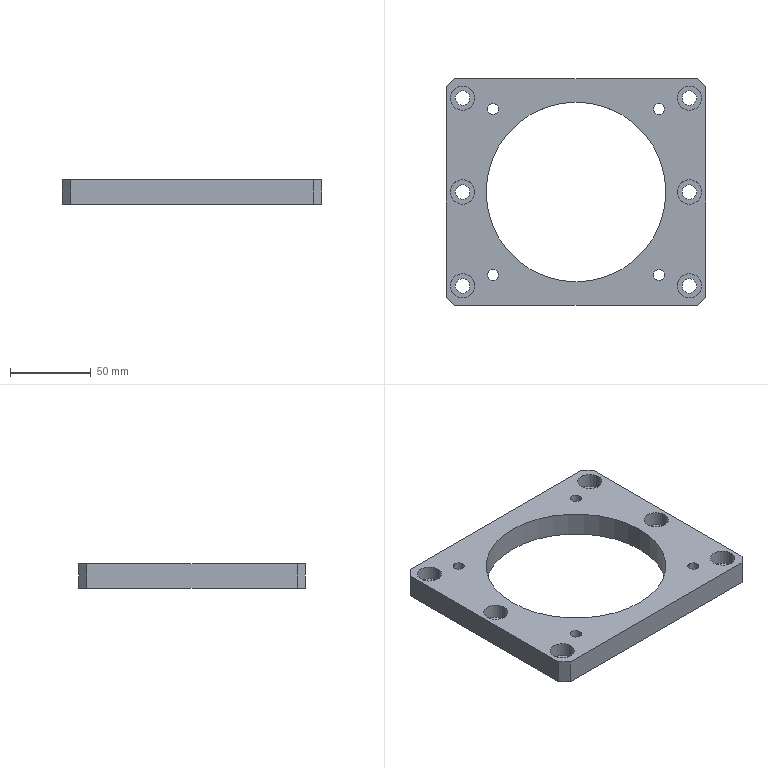Part | SolidWorks | features HoleWzd 2, CirPattern 1, Extrusion 1, MirrorPattern 1 | 1 solid | 50 faces | box 160 x 140 x 15 mm | volume 176085 mm3 | cylinder 34 | plane 16 | commonest cylinder face diameters 9 x12 15 x12 6.8 x8 111 x2
STEP:
#1=CARTESIAN_POINT('',(-77.5,58.,6.));
#2=VERTEX_POINT('',#1);
#3=CARTESIAN_POINT('',(-62.5,58.,6.));
#4=VERTEX_POINT('',#3);
#5=CARTESIAN_POINT('',(-70.,58.,6.));
#6=DIRECTION('',(0.,0.,1.));
#7=DIRECTION('',(1.,0.,0.));
#8=AXIS2_PLACEMENT_3D('',#5,#6,#7);
#9=CIRCLE('',#8,7.5);
#10=EDGE_CURVE('',#2,#4,#9,.T.);
#11=ORIENTED_EDGE('',*,*,#10,.F.);
#12=CARTESIAN_POINT('',(-77.5,58.,15.));
#13=VERTEX_POINT('',#12);
#14=CARTESIAN_POINT('',(-77.5,58.,15.));
#15=DIRECTION('',(0.,0.,1.));
#16=VECTOR('',#15,1000.);
#17=LINE('',#14,#16);
#18=EDGE_CURVE('',#2,#13,#17,.T.);
#19=ORIENTED_EDGE('',*,*,#18,.T.);
#20=CARTESIAN_POINT('',(-62.5,58.,15.));
#21=VERTEX_POINT('',#20);
#22=CARTESIAN_POINT('',(-70.,58.,15.));
#23=DIRECTION('',(0.,0.,1.));
#24=DIRECTION('',(1.,0.,0.));
#25=AXIS2_PLACEMENT_3D('',#22,#23,#24);
#26=CIRCLE('',#25,7.5);
#27=EDGE_CURVE('',#13,#21,#26,.T.);
#28=ORIENTED_EDGE('',*,*,#27,.T.);
#29=CARTESIAN_POINT('',(-62.5,58.,15.));
#30=DIRECTION('',(0.,0.,1.));
#31=VECTOR('',#30,1000.);
#32=LINE('',#29,#31);
#33=EDGE_CURVE('',#4,#21,#32,.T.);
#34=ORIENTED_EDGE('',*,*,#33,.F.);
#35=EDGE_LOOP('',(#11,#19,#28,#34));
#36=FACE_OUTER_BOUND('',#35,.T.);
#37=CARTESIAN_POINT('',(-70.,58.,15.));
#38=DIRECTION('',(0.,0.,1.));
#39=DIRECTION('',(1.,0.,0.));
#40=AXIS2_PLACEMENT_3D('',#37,#38,#39);
#41=CYLINDRICAL_SURFACE('',#40,7.5);
#42=ADVANCED_FACE('',(#36),#41,.F.);
#43=CARTESIAN_POINT('',(-74.5,58.,0.));
#44=VERTEX_POINT('',#43);
#45=CARTESIAN_POINT('',(-65.5,58.,0.));
#46=VERTEX_POINT('',#45);
#47=CARTESIAN_POINT('',(-70.,58.,0.));
#48=DIRECTION('',(0.,0.,1.));
#49=DIRECTION('',(1.,0.,0.));
#50=AXIS2_PLACEMENT_3D('',#47,#48,#49);
#51=CIRCLE('',#50,4.5);
#52=EDGE_CURVE('',#44,#46,#51,.T.);
#53=ORIENTED_EDGE('',*,*,#52,.F.);
#54=CARTESIAN_POINT('',(-74.5,58.,6.));
#55=VERTEX_POINT('',#54);
#56=CARTESIAN_POINT('',(-74.5,58.,15.));
#57=DIRECTION('',(0.,0.,1.));
#58=VECTOR('',#57,1000.);
#59=LINE('',#56,#58);
#60=EDGE_CURVE('',#44,#55,#59,.T.);
#61=ORIENTED_EDGE('',*,*,#60,.T.);
#62=CARTESIAN_POINT('',(-65.5,58.,6.));
#63=VERTEX_POINT('',#62);
#64=CARTESIAN_POINT('',(-70.,58.,6.));
#65=DIRECTION('',(0.,0.,1.));
#66=DIRECTION('',(1.,0.,0.));
#67=AXIS2_PLACEMENT_3D('',#64,#65,#66);
#68=CIRCLE('',#67,4.5);
#69=EDGE_CURVE('',#55,#63,#68,.T.);
#70=ORIENTED_EDGE('',*,*,#69,.T.);
#71=CARTESIAN_POINT('',(-65.5,58.,15.));
#72=DIRECTION('',(0.,0.,1.));
#73=VECTOR('',#72,1000.);
#74=LINE('',#71,#73);
#75=EDGE_CURVE('',#46,#63,#74,.T.);
#76=ORIENTED_EDGE('',*,*,#75,.F.);
#77=EDGE_LOOP('',(#53,#61,#70,#76));
#78=FACE_OUTER_BOUND('',#77,.T.);
#79=CARTESIAN_POINT('',(-70.,58.,15.));
#80=DIRECTION('',(0.,0.,1.));
#81=DIRECTION('',(1.,0.,0.));
#82=AXIS2_PLACEMENT_3D('',#79,#80,#81);
#83=CYLINDRICAL_SURFACE('',#82,4.5);
#84=ADVANCED_FACE('',(#78),#83,.F.);
#85=CARTESIAN_POINT('',(-77.5,0.,6.));
#86=VERTEX_POINT('',#85);
#87=CARTESIAN_POINT('',(-62.5,0.,6.));
#88=VERTEX_POINT('',#87);
#89=CARTESIAN_POINT('',(-70.,0.,6.));
#90=DIRECTION('',(0.,0.,1.));
#91=DIRECTION('',(1.,0.,0.));
#92=AXIS2_PLACEMENT_3D('',#89,#90,#91);
#93=CIRCLE('',#92,7.5);
#94=EDGE_CURVE('',#86,#88,#93,.T.);
#95=ORIENTED_EDGE('',*,*,#94,.F.);
#96=CARTESIAN_POINT('',(-77.5,0.,15.));
#97=VERTEX_POINT('',#96);
#98=CARTESIAN_POINT('',(-77.5,0.,15.));
#99=DIRECTION('',(0.,0.,1.));
#100=VECTOR('',#99,1000.);
#101=LINE('',#98,#100);
#102=EDGE_CURVE('',#86,#97,#101,.T.);
#103=ORIENTED_EDGE('',*,*,#102,.T.);
#104=CARTESIAN_POINT('',(-62.5,0.,15.));
#105=VERTEX_POINT('',#104);
#106=CARTESIAN_POINT('',(-70.,0.,15.));
#107=DIRECTION('',(0.,0.,1.));
#108=DIRECTION('',(1.,0.,0.));
#109=AXIS2_PLACEMENT_3D('',#106,#107,#108);
#110=CIRCLE('',#109,7.5);
#111=EDGE_CURVE('',#97,#105,#110,.T.);
#112=ORIENTED_EDGE('',*,*,#111,.T.);
#113=CARTESIAN_POINT('',(-62.5,0.,15.));
#114=DIRECTION('',(0.,0.,1.));
#115=VECTOR('',#114,1000.);
#116=LINE('',#113,#115);
#117=EDGE_CURVE('',#88,#105,#116,.T.);
#118=ORIENTED_EDGE('',*,*,#117,.F.);
#119=EDGE_LOOP('',(#95,#103,#112,#118));
#120=FACE_OUTER_BOUND('',#119,.T.);
#121=CARTESIAN_POINT('',(-70.,0.,15.));
#122=DIRECTION('',(0.,0.,1.));
#123=DIRECTION('',(1.,0.,0.));
#124=AXIS2_PLACEMENT_3D('',#121,#122,#123);
#125=CYLINDRICAL_SURFACE('',#124,7.5);
#126=ADVANCED_FACE('',(#120),#125,.F.);
#127=CARTESIAN_POINT('',(-74.5,0.,0.));
#128=VERTEX_POINT('',#127);
#129=CARTESIAN_POINT('',(-65.5,0.,0.));
#130=VERTEX_POINT('',#129);
#131=CARTESIAN_POINT('',(-70.,0.,0.));
#132=DIRECTION('',(0.,0.,1.));
#133=DIRECTION('',(1.,0.,0.));
#134=AXIS2_PLACEMENT_3D('',#131,#132,#133);
#135=CIRCLE('',#134,4.5);
#136=EDGE_CURVE('',#128,#130,#135,.T.);
#137=ORIENTED_EDGE('',*,*,#136,.F.);
#138=CARTESIAN_POINT('',(-74.5,0.,6.));
#139=VERTEX_POINT('',#138);
#140=CARTESIAN_POINT('',(-74.5,0.,15.));
#141=DIRECTION('',(0.,0.,1.));
#142=VECTOR('',#141,1000.);
#143=LINE('',#140,#142);
#144=EDGE_CURVE('',#128,#139,#143,.T.);
#145=ORIENTED_EDGE('',*,*,#144,.T.);
#146=CARTESIAN_POINT('',(-65.5,0.,6.));
#147=VERTEX_POINT('',#146);
#148=CARTESIAN_POINT('',(-70.,0.,6.));
#149=DIRECTION('',(0.,0.,1.));
#150=DIRECTION('',(1.,0.,0.));
#151=AXIS2_PLACEMENT_3D('',#148,#149,#150);
#152=CIRCLE('',#151,4.5);
#153=EDGE_CURVE('',#139,#147,#152,.T.);
#154=ORIENTED_EDGE('',*,*,#153,.T.);
#155=CARTESIAN_POINT('',(-65.5,0.,15.));
#156=DIRECTION('',(0.,0.,1.));
#157=VECTOR('',#156,1000.);
#158=LINE('',#155,#157);
#159=EDGE_CURVE('',#130,#147,#158,.T.);
#160=ORIENTED_EDGE('',*,*,#159,.F.);
#161=EDGE_LOOP('',(#137,#145,#154,#160));
#162=FACE_OUTER_BOUND('',#161,.T.);
#163=CARTESIAN_POINT('',(-70.,0.,15.));
#164=DIRECTION('',(0.,0.,1.));
#165=DIRECTION('',(1.,0.,0.));
#166=AXIS2_PLACEMENT_3D('',#163,#164,#165);
#167=CYLINDRICAL_SURFACE('',#166,4.5);
#168=ADVANCED_FACE('',(#162),#167,.F.);
#169=CARTESIAN_POINT('',(-77.5,-58.,6.));
#170=VERTEX_POINT('',#169);
#171=CARTESIAN_POINT('',(-62.5,-58.,6.));
#172=VERTEX_POINT('',#171);
#173=CARTESIAN_POINT('',(-70.,-58.,6.));
#174=DIRECTION('',(0.,0.,1.));
#175=DIRECTION('',(1.,0.,0.));
#176=AXIS2_PLACEMENT_3D('',#173,#174,#175);
#177=CIRCLE('',#176,7.5);
#178=EDGE_CURVE('',#170,#172,#177,.T.);
#179=ORIENTED_EDGE('',*,*,#178,.F.);
#180=CARTESIAN_POINT('',(-77.5,-58.,15.));
#181=VERTEX_POINT('',#180);
#182=CARTESIAN_POINT('',(-77.5,-58.,15.));
#183=DIRECTION('',(0.,0.,1.));
#184=VECTOR('',#183,1000.);
#185=LINE('',#182,#184);
#186=EDGE_CURVE('',#170,#181,#185,.T.);
#187=ORIENTED_EDGE('',*,*,#186,.T.);
#188=CARTESIAN_POINT('',(-62.5,-58.,15.));
#189=VERTEX_POINT('',#188);
#190=CARTESIAN_POINT('',(-70.,-58.,15.));
#191=DIRECTION('',(0.,0.,1.));
#192=DIRECTION('',(1.,0.,0.));
#193=AXIS2_PLACEMENT_3D('',#190,#191,#192);
#194=CIRCLE('',#193,7.5);
#195=EDGE_CURVE('',#181,#189,#194,.T.);
#196=ORIENTED_EDGE('',*,*,#195,.T.);
#197=CARTESIAN_POINT('',(-62.5,-58.,15.));
#198=DIRECTION('',(0.,0.,1.));
#199=VECTOR('',#198,1000.);
#200=LINE('',#197,#199);
#201=EDGE_CURVE('',#172,#189,#200,.T.);
#202=ORIENTED_EDGE('',*,*,#201,.F.);
#203=EDGE_LOOP('',(#179,#187,#196,#202));
#204=FACE_OUTER_BOUND('',#203,.T.);
#205=CARTESIAN_POINT('',(-70.,-58.,15.));
#206=DIRECTION('',(0.,0.,1.));
#207=DIRECTION('',(1.,0.,0.));
#208=AXIS2_PLACEMENT_3D('',#205,#206,#207);
#209=CYLINDRICAL_SURFACE('',#208,7.5);
#210=ADVANCED_FACE('',(#204),#209,.F.);
#211=CARTESIAN_POINT('',(-74.5,-58.,0.));
#212=VERTEX_POINT('',#211);
#213=CARTESIAN_POINT('',(-65.5,-58.,0.));
#214=VERTEX_POINT('',#213);
#215=CARTESIAN_POINT('',(-70.,-58.,0.));
#216=DIRECTION('',(0.,0.,1.));
#217=DIRECTION('',(1.,0.,0.));
#218=AXIS2_PLACEMENT_3D('',#215,#216,#217);
#219=CIRCLE('',#218,4.5);
#220=EDGE_CURVE('',#212,#214,#219,.T.);
#221=ORIENTED_EDGE('',*,*,#220,.F.);
#222=CARTESIAN_POINT('',(-74.5,-58.,6.));
#223=VERTEX_POINT('',#222);
#224=CARTESIAN_POINT('',(-74.5,-58.,15.));
#225=DIRECTION('',(0.,0.,1.));
#226=VECTOR('',#225,1000.);
#227=LINE('',#224,#226);
#228=EDGE_CURVE('',#212,#223,#227,.T.);
#229=ORIENTED_EDGE('',*,*,#228,.T.);
#230=CARTESIAN_POINT('',(-65.5,-58.,6.));
#231=VERTEX_POINT('',#230);
#232=CARTESIAN_POINT('',(-70.,-58.,6.));
#233=DIRECTION('',(0.,0.,1.));
#234=DIRECTION('',(1.,0.,0.));
#235=AXIS2_PLACEMENT_3D('',#232,#233,#234);
#236=CIRCLE('',#235,4.5);
#237=EDGE_CURVE('',#223,#231,#236,.T.);
#238=ORIENTED_EDGE('',*,*,#237,.T.);
#239=CARTESIAN_POINT('',(-65.5,-58.,15.));
#240=DIRECTION('',(0.,0.,1.));
#241=VECTOR('',#240,1000.);
#242=LINE('',#239,#241);
#243=EDGE_CURVE('',#214,#231,#242,.T.);
#244=ORIENTED_EDGE('',*,*,#243,.F.);
#245=EDGE_LOOP('',(#221,#229,#238,#244));
#246=FACE_OUTER_BOUND('',#245,.T.);
#247=CARTESIAN_POINT('',(-70.,-58.,15.));
#248=DIRECTION('',(0.,0.,1.));
#249=DIRECTION('',(1.,0.,0.));
#250=AXIS2_PLACEMENT_3D('',#247,#248,#249);
#251=CYLINDRICAL_SURFACE('',#250,4.5);
#252=ADVANCED_FACE('',(#246),#251,.F.);
#253=CARTESIAN_POINT('',(62.5,58.,6.));
#254=VERTEX_POINT('',#253);
#255=CARTESIAN_POINT('',(77.5,58.,6.));
#256=VERTEX_POINT('',#255);
#257=CARTESIAN_POINT('',(70.,58.,6.));
#258=DIRECTION('',(0.,0.,1.));
#259=DIRECTION('',(1.,0.,0.));
#260=AXIS2_PLACEMENT_3D('',#257,#258,#259);
#261=CIRCLE('',#260,7.5);
#262=EDGE_CURVE('',#254,#256,#261,.T.);
#263=ORIENTED_EDGE('',*,*,#262,.F.);
#264=CARTESIAN_POINT('',(62.5,58.,15.));
#265=VERTEX_POINT('',#264);
#266=CARTESIAN_POINT('',(62.5,58.,15.));
#267=DIRECTION('',(0.,0.,1.));
#268=VECTOR('',#267,1000.);
#269=LINE('',#266,#268);
#270=EDGE_CURVE('',#254,#265,#269,.T.);
#271=ORIENTED_EDGE('',*,*,#270,.T.);
#272=CARTESIAN_POINT('',(77.5,58.,15.));
#273=VERTEX_POINT('',#272);
#274=CARTESIAN_POINT('',(70.,58.,15.));
#275=DIRECTION('',(0.,0.,1.));
#276=DIRECTION('',(1.,0.,0.));
#277=AXIS2_PLACEMENT_3D('',#274,#275,#276);
#278=CIRCLE('',#277,7.5);
#279=EDGE_CURVE('',#265,#273,#278,.T.);
#280=ORIENTED_EDGE('',*,*,#279,.T.);
#281=CARTESIAN_POINT('',(77.5,58.,15.));
#282=DIRECTION('',(0.,0.,1.));
#283=VECTOR('',#282,1000.);
#284=LINE('',#281,#283);
#285=EDGE_CURVE('',#256,#273,#284,.T.);
#286=ORIENTED_EDGE('',*,*,#285,.F.);
#287=EDGE_LOOP('',(#263,#271,#280,#286));
#288=FACE_OUTER_BOUND('',#287,.T.);
#289=CARTESIAN_POINT('',(70.,58.,15.));
#290=DIRECTION('',(0.,0.,1.));
#291=DIRECTION('',(1.,0.,0.));
#292=AXIS2_PLACEMENT_3D('',#289,#290,#291);
#293=CYLINDRICAL_SURFACE('',#292,7.5);
#294=ADVANCED_FACE('',(#288),#293,.F.);
#295=CARTESIAN_POINT('',(65.5,58.,0.));
#296=VERTEX_POINT('',#295);
#297=CARTESIAN_POINT('',(74.5,58.,0.));
#298=VERTEX_POINT('',#297);
#299=CARTESIAN_POINT('',(70.,58.,0.));
#300=DIRECTION('',(0.,0.,1.));
#301=DIRECTION('',(1.,0.,0.));
#302=AXIS2_PLACEMENT_3D('',#299,#300,#301);
#303=CIRCLE('',#302,4.5);
#304=EDGE_CURVE('',#296,#298,#303,.T.);
#305=ORIENTED_EDGE('',*,*,#304,.F.);
#306=CARTESIAN_POINT('',(65.5,58.,6.));
#307=VERTEX_POINT('',#306);
#308=CARTESIAN_POINT('',(65.5,58.,15.));
#309=DIRECTION('',(0.,0.,1.));
#310=VECTOR('',#309,1000.);
#311=LINE('',#308,#310);
#312=EDGE_CURVE('',#296,#307,#311,.T.);
#313=ORIENTED_EDGE('',*,*,#312,.T.);
#314=CARTESIAN_POINT('',(74.5,58.,6.));
#315=VERTEX_POINT('',#314);
#316=CARTESIAN_POINT('',(70.,58.,6.));
#317=DIRECTION('',(0.,0.,1.));
#318=DIRECTION('',(1.,0.,0.));
#319=AXIS2_PLACEMENT_3D('',#316,#317,#318);
#320=CIRCLE('',#319,4.5);
#321=EDGE_CURVE('',#307,#315,#320,.T.);
#322=ORIENTED_EDGE('',*,*,#321,.T.);
#323=CARTESIAN_POINT('',(74.5,58.,15.));
#324=DIRECTION('',(0.,0.,1.));
#325=VECTOR('',#324,1000.);
#326=LINE('',#323,#325);
#327=EDGE_CURVE('',#298,#315,#326,.T.);
#328=ORIENTED_EDGE('',*,*,#327,.F.);
#329=EDGE_LOOP('',(#305,#313,#322,#328));
#330=FACE_OUTER_BOUND('',#329,.T.);
#331=CARTESIAN_POINT('',(70.,58.,15.));
#332=DIRECTION('',(0.,0.,1.));
#333=DIRECTION('',(1.,0.,0.));
#334=AXIS2_PLACEMENT_3D('',#331,#332,#333);
#335=CYLINDRICAL_SURFACE('',#334,4.5);
#336=ADVANCED_FACE('',(#330),#335,.F.);
#337=CARTESIAN_POINT('',(62.5,0.,6.));
#338=VERTEX_POINT('',#337);
#339=CARTESIAN_POINT('',(77.5,0.,6.));
#340=VERTEX_POINT('',#339);
#341=CARTESIAN_POINT('',(70.,0.,6.));
#342=DIRECTION('',(0.,0.,1.));
#343=DIRECTION('',(1.,0.,0.));
#344=AXIS2_PLACEMENT_3D('',#341,#342,#343);
#345=CIRCLE('',#344,7.5);
#346=EDGE_CURVE('',#338,#340,#345,.T.);
#347=ORIENTED_EDGE('',*,*,#346,.F.);
#348=CARTESIAN_POINT('',(62.5,0.,15.));
#349=VERTEX_POINT('',#348);
#350=CARTESIAN_POINT('',(62.5,0.,15.));
#351=DIRECTION('',(0.,0.,1.));
#352=VECTOR('',#351,1000.);
#353=LINE('',#350,#352);
#354=EDGE_CURVE('',#338,#349,#353,.T.);
#355=ORIENTED_EDGE('',*,*,#354,.T.);
#356=CARTESIAN_POINT('',(77.5,0.,15.));
#357=VERTEX_POINT('',#356);
#358=CARTESIAN_POINT('',(70.,0.,15.));
#359=DIRECTION('',(0.,0.,1.));
#360=DIRECTION('',(1.,0.,0.));
#361=AXIS2_PLACEMENT_3D('',#358,#359,#360);
#362=CIRCLE('',#361,7.5);
#363=EDGE_CURVE('',#349,#357,#362,.T.);
#364=ORIENTED_EDGE('',*,*,#363,.T.);
#365=CARTESIAN_POINT('',(77.5,0.,15.));
#366=DIRECTION('',(0.,0.,1.));
#367=VECTOR('',#366,1000.);
#368=LINE('',#365,#367);
#369=EDGE_CURVE('',#340,#357,#368,.T.);
#370=ORIENTED_EDGE('',*,*,#369,.F.);
#371=EDGE_LOOP('',(#347,#355,#364,#370));
#372=FACE_OUTER_BOUND('',#371,.T.);
#373=CARTESIAN_POINT('',(70.,0.,15.));
#374=DIRECTION('',(0.,0.,1.));
#375=DIRECTION('',(1.,0.,0.));
#376=AXIS2_PLACEMENT_3D('',#373,#374,#375);
#377=CYLINDRICAL_SURFACE('',#376,7.5);
#378=ADVANCED_FACE('',(#372),#377,.F.);
#379=CARTESIAN_POINT('',(65.5,0.,0.));
#380=VERTEX_POINT('',#379);
#381=CARTESIAN_POINT('',(74.5,0.,0.));
#382=VERTEX_POINT('',#381);
#383=CARTESIAN_POINT('',(70.,0.,0.));
#384=DIRECTION('',(0.,0.,1.));
#385=DIRECTION('',(1.,0.,0.));
#386=AXIS2_PLACEMENT_3D('',#383,#384,#385);
#387=CIRCLE('',#386,4.5);
#388=EDGE_CURVE('',#380,#382,#387,.T.);
#389=ORIENTED_EDGE('',*,*,#388,.F.);
#390=CARTESIAN_POINT('',(65.5,0.,6.));
#391=VERTEX_POINT('',#390);
#392=CARTESIAN_POINT('',(65.5,0.,15.));
#393=DIRECTION('',(0.,0.,1.));
#394=VECTOR('',#393,1000.);
#395=LINE('',#392,#394);
#396=EDGE_CURVE('',#380,#391,#395,.T.);
#397=ORIENTED_EDGE('',*,*,#396,.T.);
#398=CARTESIAN_POINT('',(74.5,0.,6.));
#399=VERTEX_POINT('',#398);
#400=CARTESIAN_POINT('',(70.,0.,6.));
#401=DIRECTION('',(0.,0.,1.));
#402=DIRECTION('',(1.,0.,0.));
#403=AXIS2_PLACEMENT_3D('',#400,#401,#402);
#404=CIRCLE('',#403,4.5);
#405=EDGE_CURVE('',#391,#399,#404,.T.);
#406=ORIENTED_EDGE('',*,*,#405,.T.);
#407=CARTESIAN_POINT('',(74.5,0.,15.));
#408=DIRECTION('',(0.,0.,1.));
#409=VECTOR('',#408,1000.);
#410=LINE('',#407,#409);
#411=EDGE_CURVE('',#382,#399,#410,.T.);
#412=ORIENTED_EDGE('',*,*,#411,.F.);
#413=EDGE_LOOP('',(#389,#397,#406,#412));
#414=FACE_OUTER_BOUND('',#413,.T.);
#415=CARTESIAN_POINT('',(70.,0.,15.));
#416=DIRECTION('',(0.,0.,1.));
#417=DIRECTION('',(1.,0.,0.));
#418=AXIS2_PLACEMENT_3D('',#415,#416,#417);
#419=CYLINDRICAL_SURFACE('',#418,4.5);
#420=ADVANCED_FACE('',(#414),#419,.F.);
#421=CARTESIAN_POINT('',(62.5,-58.,6.));
#422=VERTEX_POINT('',#421);
#423=CARTESIAN_POINT('',(77.5,-58.,6.));
#424=VERTEX_POINT('',#423);
#425=CARTESIAN_POINT('',(70.,-58.,6.));
#426=DIRECTION('',(0.,0.,1.));
#427=DIRECTION('',(1.,0.,0.));
#428=AXIS2_PLACEMENT_3D('',#425,#426,#427);
#429=CIRCLE('',#428,7.5);
#430=EDGE_CURVE('',#422,#424,#429,.T.);
#431=ORIENTED_EDGE('',*,*,#430,.F.);
#432=CARTESIAN_POINT('',(62.5,-58.,15.));
#433=VERTEX_POINT('',#432);
#434=CARTESIAN_POINT('',(62.5,-58.,15.));
#435=DIRECTION('',(0.,0.,1.));
#436=VECTOR('',#435,1000.);
#437=LINE('',#434,#436);
#438=EDGE_CURVE('',#422,#433,#437,.T.);
#439=ORIENTED_EDGE('',*,*,#438,.T.);
#440=CARTESIAN_POINT('',(77.5,-58.,15.));
#441=VERTEX_POINT('',#440);
#442=CARTESIAN_POINT('',(70.,-58.,15.));
#443=DIRECTION('',(0.,0.,1.));
#444=DIRECTION('',(1.,0.,0.));
#445=AXIS2_PLACEMENT_3D('',#442,#443,#444);
#446=CIRCLE('',#445,7.5);
#447=EDGE_CURVE('',#433,#441,#446,.T.);
#448=ORIENTED_EDGE('',*,*,#447,.T.);
#449=CARTESIAN_POINT('',(77.5,-58.,15.));
#450=DIRECTION('',(0.,0.,1.));
#451=VECTOR('',#450,1000.);
#452=LINE('',#449,#451);
#453=EDGE_CURVE('',#424,#441,#452,.T.);
#454=ORIENTED_EDGE('',*,*,#453,.F.);
#455=EDGE_LOOP('',(#431,#439,#448,#454));
#456=FACE_OUTER_BOUND('',#455,.T.);
#457=CARTESIAN_POINT('',(70.,-58.,15.));
#458=DIRECTION('',(0.,0.,1.));
#459=DIRECTION('',(1.,0.,0.));
#460=AXIS2_PLACEMENT_3D('',#457,#458,#459);
#461=CYLINDRICAL_SURFACE('',#460,7.5);
#462=ADVANCED_FACE('',(#456),#461,.F.);
#463=CARTESIAN_POINT('',(65.5,-58.,0.));
#464=VERTEX_POINT('',#463);
#465=CARTESIAN_POINT('',(74.5,-58.,0.));
#466=VERTEX_POINT('',#465);
#467=CARTESIAN_POINT('',(70.,-58.,0.));
#468=DIRECTION('',(0.,0.,1.));
#469=DIRECTION('',(1.,0.,0.));
#470=AXIS2_PLACEMENT_3D('',#467,#468,#469);
#471=CIRCLE('',#470,4.5);
#472=EDGE_CURVE('',#464,#466,#471,.T.);
#473=ORIENTED_EDGE('',*,*,#472,.F.);
#474=CARTESIAN_POINT('',(65.5,-58.,6.));
#475=VERTEX_POINT('',#474);
#476=CARTESIAN_POINT('',(65.5,-58.,15.));
#477=DIRECTION('',(0.,0.,1.));
#478=VECTOR('',#477,1000.);
#479=LINE('',#476,#478);
#480=EDGE_CURVE('',#464,#475,#479,.T.);
#481=ORIENTED_EDGE('',*,*,#480,.T.);
#482=CARTESIAN_POINT('',(74.5,-58.,6.));
#483=VERTEX_POINT('',#482);
#484=CARTESIAN_POINT('',(70.,-58.,6.));
#485=DIRECTION('',(0.,0.,1.));
#486=DIRECTION('',(1.,0.,0.));
#487=AXIS2_PLACEMENT_3D('',#484,#485,#486);
#488=CIRCLE('',#487,4.5);
#489=EDGE_CURVE('',#475,#483,#488,.T.);
#490=ORIENTED_EDGE('',*,*,#489,.T.);
#491=CARTESIAN_POINT('',(74.5,-58.,15.));
#492=DIRECTION('',(0.,0.,1.));
#493=VECTOR('',#492,1000.);
#494=LINE('',#491,#493);
#495=EDGE_CURVE('',#466,#483,#494,.T.);
#496=ORIENTED_EDGE('',*,*,#495,.F.);
#497=EDGE_LOOP('',(#473,#481,#490,#496));
#498=FACE_OUTER_BOUND('',#497,.T.);
#499=CARTESIAN_POINT('',(70.,-58.,15.));
#500=DIRECTION('',(0.,0.,1.));
#501=DIRECTION('',(1.,0.,0.));
#502=AXIS2_PLACEMENT_3D('',#499,#500,#501);
#503=CYLINDRICAL_SURFACE('',#502,4.5);
#504=ADVANCED_FACE('',(#498),#503,.F.);
#505=CARTESIAN_POINT('',(51.265,-47.865,0.));
#506=VERTEX_POINT('',#505);
#507=CARTESIAN_POINT('',(51.265,-54.665,0.));
#508=VERTEX_POINT('',#507);
#509=CARTESIAN_POINT('',(51.265,-51.265,0.));
#510=DIRECTION('',(0.,0.,1.));
#511=DIRECTION('',(0.,-1.,0.));
#512=AXIS2_PLACEMENT_3D('',#509,#510,#511);
#513=CIRCLE('',#512,3.4);
#514=EDGE_CURVE('',#506,#508,#513,.T.);
#515=ORIENTED_EDGE('',*,*,#514,.F.);
#516=CARTESIAN_POINT('',(51.265,-47.865,15.));
#517=VERTEX_POINT('',#516);
#518=CARTESIAN_POINT('',(51.265,-47.865,15.));
#519=DIRECTION('',(0.,0.,1.));
#520=VECTOR('',#519,1000.);
#521=LINE('',#518,#520);
#522=EDGE_CURVE('',#506,#517,#521,.T.);
#523=ORIENTED_EDGE('',*,*,#522,.T.);
#524=CARTESIAN_POINT('',(51.265,-54.665,15.));
#525=VERTEX_POINT('',#524);
#526=CARTESIAN_POINT('',(51.265,-51.265,15.));
#527=DIRECTION('',(0.,0.,1.));
#528=DIRECTION('',(0.,-1.,0.));
#529=AXIS2_PLACEMENT_3D('',#526,#527,#528);
#530=CIRCLE('',#529,3.4);
#531=EDGE_CURVE('',#517,#525,#530,.T.);
#532=ORIENTED_EDGE('',*,*,#531,.T.);
#533=CARTESIAN_POINT('',(51.265,-54.665,15.));
#534=DIRECTION('',(0.,0.,1.));
#535=VECTOR('',#534,1000.);
#536=LINE('',#533,#535);
#537=EDGE_CURVE('',#508,#525,#536,.T.);
#538=ORIENTED_EDGE('',*,*,#537,.F.);
#539=EDGE_LOOP('',(#515,#523,#532,#538));
#540=FACE_OUTER_BOUND('',#539,.T.);
#541=CARTESIAN_POINT('',(51.265,-51.265,15.));
#542=DIRECTION('',(0.,0.,1.));
#543=DIRECTION('',(0.,-1.,0.));
#544=AXIS2_PLACEMENT_3D('',#541,#542,#543);
#545=CYLINDRICAL_SURFACE('',#544,3.4);
#546=ADVANCED_FACE('',(#540),#545,.F.);
#547=CARTESIAN_POINT('',(-47.865,-51.265,0.));
#548=VERTEX_POINT('',#547);
#549=CARTESIAN_POINT('',(-54.665,-51.265,0.));
#550=VERTEX_POINT('',#549);
#551=CARTESIAN_POINT('',(-51.265,-51.265,0.));
#552=DIRECTION('',(0.,0.,1.));
#553=DIRECTION('',(-1.,0.,0.));
#554=AXIS2_PLACEMENT_3D('',#551,#552,#553);
#555=CIRCLE('',#554,3.4);
#556=EDGE_CURVE('',#548,#550,#555,.T.);
#557=ORIENTED_EDGE('',*,*,#556,.F.);
#558=CARTESIAN_POINT('',(-47.865,-51.265,15.));
#559=VERTEX_POINT('',#558);
#560=CARTESIAN_POINT('',(-47.865,-51.265,15.));
#561=DIRECTION('',(0.,0.,1.));
#562=VECTOR('',#561,1000.);
#563=LINE('',#560,#562);
#564=EDGE_CURVE('',#548,#559,#563,.T.);
#565=ORIENTED_EDGE('',*,*,#564,.T.);
#566=CARTESIAN_POINT('',(-54.665,-51.265,15.));
#567=VERTEX_POINT('',#566);
#568=CARTESIAN_POINT('',(-51.265,-51.265,15.));
#569=DIRECTION('',(0.,0.,1.));
#570=DIRECTION('',(-1.,0.,0.));
#571=AXIS2_PLACEMENT_3D('',#568,#569,#570);
#572=CIRCLE('',#571,3.4);
#573=EDGE_CURVE('',#559,#567,#572,.T.);
#574=ORIENTED_EDGE('',*,*,#573,.T.);
#575=CARTESIAN_POINT('',(-54.665,-51.265,15.));
#576=DIRECTION('',(0.,0.,1.));
#577=VECTOR('',#576,1000.);
#578=LINE('',#575,#577);
#579=EDGE_CURVE('',#550,#567,#578,.T.);
#580=ORIENTED_EDGE('',*,*,#579,.F.);
#581=EDGE_LOOP('',(#557,#565,#574,#580));
#582=FACE_OUTER_BOUND('',#581,.T.);
#583=CARTESIAN_POINT('',(-51.265,-51.265,15.));
#584=DIRECTION('',(0.,0.,1.));
#585=DIRECTION('',(-1.,0.,0.));
#586=AXIS2_PLACEMENT_3D('',#583,#584,#585);
#587=CYLINDRICAL_SURFACE('',#586,3.4);
#588=ADVANCED_FACE('',(#582),#587,.F.);
#589=CARTESIAN_POINT('',(-51.265,47.865,0.));
#590=VERTEX_POINT('',#589);
#591=CARTESIAN_POINT('',(-51.265,54.665,0.));
#592=VERTEX_POINT('',#591);
#593=CARTESIAN_POINT('',(-51.265,51.265,0.));
#594=DIRECTION('',(0.,0.,1.));
#595=DIRECTION('',(0.,1.,0.));
#596=AXIS2_PLACEMENT_3D('',#593,#594,#595);
#597=CIRCLE('',#596,3.4);
#598=EDGE_CURVE('',#590,#592,#597,.T.);
#599=ORIENTED_EDGE('',*,*,#598,.F.);
#600=CARTESIAN_POINT('',(-51.265,47.865,15.));
#601=VERTEX_POINT('',#600);
#602=CARTESIAN_POINT('',(-51.265,47.865,15.));
#603=DIRECTION('',(0.,0.,1.));
#604=VECTOR('',#603,1000.);
#605=LINE('',#602,#604);
#606=EDGE_CURVE('',#590,#601,#605,.T.);
#607=ORIENTED_EDGE('',*,*,#606,.T.);
#608=CARTESIAN_POINT('',(-51.265,54.665,15.));
#609=VERTEX_POINT('',#608);
#610=CARTESIAN_POINT('',(-51.265,51.265,15.));
#611=DIRECTION('',(0.,0.,1.));
#612=DIRECTION('',(0.,1.,0.));
#613=AXIS2_PLACEMENT_3D('',#610,#611,#612);
#614=CIRCLE('',#613,3.4);
#615=EDGE_CURVE('',#601,#609,#614,.T.);
#616=ORIENTED_EDGE('',*,*,#615,.T.);
#617=CARTESIAN_POINT('',(-51.265,54.665,15.));
#618=DIRECTION('',(0.,0.,1.));
#619=VECTOR('',#618,1000.);
#620=LINE('',#617,#619);
#621=EDGE_CURVE('',#592,#609,#620,.T.);
#622=ORIENTED_EDGE('',*,*,#621,.F.);
#623=EDGE_LOOP('',(#599,#607,#616,#622));
#624=FACE_OUTER_BOUND('',#623,.T.);
#625=CARTESIAN_POINT('',(-51.265,51.265,15.));
#626=DIRECTION('',(0.,0.,1.));
#627=DIRECTION('',(0.,1.,0.));
#628=AXIS2_PLACEMENT_3D('',#625,#626,#627);
#629=CYLINDRICAL_SURFACE('',#628,3.4);
#630=ADVANCED_FACE('',(#624),#629,.F.);
#631=CARTESIAN_POINT('',(47.865,51.265,0.));
#632=VERTEX_POINT('',#631);
#633=CARTESIAN_POINT('',(54.665,51.265,0.));
#634=VERTEX_POINT('',#633);
#635=CARTESIAN_POINT('',(51.265,51.265,0.));
#636=DIRECTION('',(0.,0.,1.));
#637=DIRECTION('',(1.,0.,0.));
#638=AXIS2_PLACEMENT_3D('',#635,#636,#637);
#639=CIRCLE('',#638,3.4);
#640=EDGE_CURVE('',#632,#634,#639,.T.);
#641=ORIENTED_EDGE('',*,*,#640,.F.);
#642=CARTESIAN_POINT('',(47.865,51.265,15.));
#643=VERTEX_POINT('',#642);
#644=CARTESIAN_POINT('',(47.865,51.265,15.));
#645=DIRECTION('',(0.,0.,1.));
#646=VECTOR('',#645,1000.);
#647=LINE('',#644,#646);
#648=EDGE_CURVE('',#632,#643,#647,.T.);
#649=ORIENTED_EDGE('',*,*,#648,.T.);
#650=CARTESIAN_POINT('',(54.665,51.265,15.));
#651=VERTEX_POINT('',#650);
#652=CARTESIAN_POINT('',(51.265,51.265,15.));
#653=DIRECTION('',(0.,0.,1.));
#654=DIRECTION('',(1.,0.,0.));
#655=AXIS2_PLACEMENT_3D('',#652,#653,#654);
#656=CIRCLE('',#655,3.4);
#657=EDGE_CURVE('',#643,#651,#656,.T.);
#658=ORIENTED_EDGE('',*,*,#657,.T.);
#659=CARTESIAN_POINT('',(54.665,51.265,15.));
#660=DIRECTION('',(0.,0.,1.));
#661=VECTOR('',#660,1000.);
#662=LINE('',#659,#661);
#663=EDGE_CURVE('',#634,#651,#662,.T.);
#664=ORIENTED_EDGE('',*,*,#663,.F.);
#665=EDGE_LOOP('',(#641,#649,#658,#664));
#666=FACE_OUTER_BOUND('',#665,.T.);
#667=CARTESIAN_POINT('',(51.265,51.265,15.));
#668=DIRECTION('',(0.,0.,1.));
#669=DIRECTION('',(1.,0.,0.));
#670=AXIS2_PLACEMENT_3D('',#667,#668,#669);
#671=CYLINDRICAL_SURFACE('',#670,3.4);
#672=ADVANCED_FACE('',(#666),#671,.F.);
#673=CARTESIAN_POINT('',(-55.5,0.,15.));
#674=VERTEX_POINT('',#673);
#675=CARTESIAN_POINT('',(55.5,0.,15.));
#676=VERTEX_POINT('',#675);
#677=CARTESIAN_POINT('',(0.,0.,15.));
#678=DIRECTION('',(0.,0.,1.));
#679=DIRECTION('',(1.,0.,0.));
#680=AXIS2_PLACEMENT_3D('',#677,#678,#679);
#681=CIRCLE('',#680,55.5);
#682=EDGE_CURVE('',#674,#676,#681,.T.);
#683=ORIENTED_EDGE('',*,*,#682,.T.);
#684=CARTESIAN_POINT('',(55.5,0.,0.));
#685=VERTEX_POINT('',#684);
#686=CARTESIAN_POINT('',(55.5,0.,15.));
#687=DIRECTION('',(0.,0.,-1.));
#688=VECTOR('',#687,1000.);
#689=LINE('',#686,#688);
#690=EDGE_CURVE('',#676,#685,#689,.T.);
#691=ORIENTED_EDGE('',*,*,#690,.T.);
#692=CARTESIAN_POINT('',(-55.5,0.,0.));
#693=VERTEX_POINT('',#692);
#694=CARTESIAN_POINT('',(0.,0.,0.));
#695=DIRECTION('',(0.,0.,1.));
#696=DIRECTION('',(1.,0.,0.));
#697=AXIS2_PLACEMENT_3D('',#694,#695,#696);
#698=CIRCLE('',#697,55.5);
#699=EDGE_CURVE('',#693,#685,#698,.T.);
#700=ORIENTED_EDGE('',*,*,#699,.F.);
#701=CARTESIAN_POINT('',(-55.5,0.,15.));
#702=DIRECTION('',(0.,0.,-1.));
#703=VECTOR('',#702,1000.);
#704=LINE('',#701,#703);
#705=EDGE_CURVE('',#674,#693,#704,.T.);
#706=ORIENTED_EDGE('',*,*,#705,.F.);
#707=EDGE_LOOP('',(#683,#691,#700,#706));
#708=FACE_OUTER_BOUND('',#707,.T.);
#709=CARTESIAN_POINT('',(0.,0.,15.));
#710=DIRECTION('',(0.,0.,-1.));
#711=DIRECTION('',(-1.,0.,0.));
#712=AXIS2_PLACEMENT_3D('',#709,#710,#711);
#713=CYLINDRICAL_SURFACE('',#712,55.5);
#714=ADVANCED_FACE('',(#708),#713,.F.);
#715=CARTESIAN_POINT('',(-70.,58.,15.));
#716=DIRECTION('',(0.,0.,1.));
#717=DIRECTION('',(1.,0.,0.));
#718=AXIS2_PLACEMENT_3D('',#715,#716,#717);
#719=CIRCLE('',#718,7.5);
#720=EDGE_CURVE('',#21,#13,#719,.T.);
#721=ORIENTED_EDGE('',*,*,#720,.F.);
#722=ORIENTED_EDGE('',*,*,#27,.F.);
#723=EDGE_LOOP('',(#721,#722));
#724=FACE_BOUND('',#723,.T.);
#725=CARTESIAN_POINT('',(-70.,0.,15.));
#726=DIRECTION('',(0.,0.,1.));
#727=DIRECTION('',(1.,0.,0.));
#728=AXIS2_PLACEMENT_3D('',#725,#726,#727);
#729=CIRCLE('',#728,7.5);
#730=EDGE_CURVE('',#105,#97,#729,.T.);
#731=ORIENTED_EDGE('',*,*,#730,.F.);
#732=ORIENTED_EDGE('',*,*,#111,.F.);
#733=EDGE_LOOP('',(#731,#732));
#734=FACE_BOUND('',#733,.T.);
#735=CARTESIAN_POINT('',(-70.,-58.,15.));
#736=DIRECTION('',(0.,0.,1.));
#737=DIRECTION('',(1.,0.,0.));
#738=AXIS2_PLACEMENT_3D('',#735,#736,#737);
#739=CIRCLE('',#738,7.5);
#740=EDGE_CURVE('',#189,#181,#739,.T.);
#741=ORIENTED_EDGE('',*,*,#740,.F.);
#742=ORIENTED_EDGE('',*,*,#195,.F.);
#743=EDGE_LOOP('',(#741,#742));
#744=FACE_BOUND('',#743,.T.);
#745=CARTESIAN_POINT('',(70.,58.,15.));
#746=DIRECTION('',(0.,0.,1.));
#747=DIRECTION('',(1.,0.,0.));
#748=AXIS2_PLACEMENT_3D('',#745,#746,#747);
#749=CIRCLE('',#748,7.5);
#750=EDGE_CURVE('',#273,#265,#749,.T.);
#751=ORIENTED_EDGE('',*,*,#750,.F.);
#752=ORIENTED_EDGE('',*,*,#279,.F.);
#753=EDGE_LOOP('',(#751,#752));
#754=FACE_BOUND('',#753,.T.);
#755=CARTESIAN_POINT('',(70.,0.,15.));
#756=DIRECTION('',(0.,0.,1.));
#757=DIRECTION('',(1.,0.,0.));
#758=AXIS2_PLACEMENT_3D('',#755,#756,#757);
#759=CIRCLE('',#758,7.5);
#760=EDGE_CURVE('',#357,#349,#759,.T.);
#761=ORIENTED_EDGE('',*,*,#760,.F.);
#762=ORIENTED_EDGE('',*,*,#363,.F.);
#763=EDGE_LOOP('',(#761,#762));
#764=FACE_BOUND('',#763,.T.);
#765=CARTESIAN_POINT('',(70.,-58.,15.));
#766=DIRECTION('',(0.,0.,1.));
#767=DIRECTION('',(1.,0.,0.));
#768=AXIS2_PLACEMENT_3D('',#765,#766,#767);
#769=CIRCLE('',#768,7.5);
#770=EDGE_CURVE('',#441,#433,#769,.T.);
#771=ORIENTED_EDGE('',*,*,#770,.F.);
#772=ORIENTED_EDGE('',*,*,#447,.F.);
#773=EDGE_LOOP('',(#771,#772));
#774=FACE_BOUND('',#773,.T.);
#775=CARTESIAN_POINT('',(51.265,-51.265,15.));
#776=DIRECTION('',(0.,0.,1.));
#777=DIRECTION('',(0.,-1.,0.));
#778=AXIS2_PLACEMENT_3D('',#775,#776,#777);
#779=CIRCLE('',#778,3.4);
#780=EDGE_CURVE('',#525,#517,#779,.T.);
#781=ORIENTED_EDGE('',*,*,#780,.F.);
#782=ORIENTED_EDGE('',*,*,#531,.F.);
#783=EDGE_LOOP('',(#781,#782));
#784=FACE_BOUND('',#783,.T.);
#785=CARTESIAN_POINT('',(-51.265,-51.265,15.));
#786=DIRECTION('',(0.,0.,1.));
#787=DIRECTION('',(-1.,0.,0.));
#788=AXIS2_PLACEMENT_3D('',#785,#786,#787);
#789=CIRCLE('',#788,3.4);
#790=EDGE_CURVE('',#567,#559,#789,.T.);
#791=ORIENTED_EDGE('',*,*,#790,.F.);
#792=ORIENTED_EDGE('',*,*,#573,.F.);
#793=EDGE_LOOP('',(#791,#792));
#794=FACE_BOUND('',#793,.T.);
#795=CARTESIAN_POINT('',(-51.265,51.265,15.));
#796=DIRECTION('',(0.,0.,1.));
#797=DIRECTION('',(0.,1.,0.));
#798=AXIS2_PLACEMENT_3D('',#795,#796,#797);
#799=CIRCLE('',#798,3.4);
#800=EDGE_CURVE('',#609,#601,#799,.T.);
#801=ORIENTED_EDGE('',*,*,#800,.F.);
#802=ORIENTED_EDGE('',*,*,#615,.F.);
#803=EDGE_LOOP('',(#801,#802));
#804=FACE_BOUND('',#803,.T.);
#805=CARTESIAN_POINT('',(51.265,51.265,15.));
#806=DIRECTION('',(0.,0.,1.));
#807=DIRECTION('',(1.,0.,0.));
#808=AXIS2_PLACEMENT_3D('',#805,#806,#807);
#809=CIRCLE('',#808,3.4);
#810=EDGE_CURVE('',#651,#643,#809,.T.);
#811=ORIENTED_EDGE('',*,*,#810,.F.);
#812=ORIENTED_EDGE('',*,*,#657,.F.);
#813=EDGE_LOOP('',(#811,#812));
#814=FACE_BOUND('',#813,.T.);
#815=CARTESIAN_POINT('',(75.,70.,15.));
#816=VERTEX_POINT('',#815);
#817=CARTESIAN_POINT('',(-75.,70.,15.));
#818=VERTEX_POINT('',#817);
#819=CARTESIAN_POINT('',(-75.,70.,15.));
#820=DIRECTION('',(-1.,0.,0.));
#821=VECTOR('',#820,1000.);
#822=LINE('',#819,#821);
#823=EDGE_CURVE('',#816,#818,#822,.T.);
#824=ORIENTED_EDGE('',*,*,#823,.T.);
#825=CARTESIAN_POINT('',(-80.,65.,15.));
#826=VERTEX_POINT('',#825);
#827=CARTESIAN_POINT('',(-80.,65.,15.));
#828=DIRECTION('',(-0.7071,-0.7071,0.));
#829=VECTOR('',#828,1000.);
#830=LINE('',#827,#829);
#831=EDGE_CURVE('',#818,#826,#830,.T.);
#832=ORIENTED_EDGE('',*,*,#831,.T.);
#833=CARTESIAN_POINT('',(-80.,-65.,15.));
#834=VERTEX_POINT('',#833);
#835=CARTESIAN_POINT('',(-80.,-65.,15.));
#836=DIRECTION('',(0.,-1.,0.));
#837=VECTOR('',#836,1000.);
#838=LINE('',#835,#837);
#839=EDGE_CURVE('',#826,#834,#838,.T.);
#840=ORIENTED_EDGE('',*,*,#839,.T.);
#841=CARTESIAN_POINT('',(-75.,-70.,15.));
#842=VERTEX_POINT('',#841);
#843=CARTESIAN_POINT('',(-80.,-65.,15.));
#844=DIRECTION('',(0.7071,-0.7071,0.));
#845=VECTOR('',#844,1000.);
#846=LINE('',#843,#845);
#847=EDGE_CURVE('',#834,#842,#846,.T.);
#848=ORIENTED_EDGE('',*,*,#847,.T.);
#849=CARTESIAN_POINT('',(75.,-70.,15.));
#850=VERTEX_POINT('',#849);
#851=CARTESIAN_POINT('',(-75.,-70.,15.));
#852=DIRECTION('',(1.,0.,0.));
#853=VECTOR('',#852,1000.);
#854=LINE('',#851,#853);
#855=EDGE_CURVE('',#842,#850,#854,.T.);
#856=ORIENTED_EDGE('',*,*,#855,.T.);
#857=CARTESIAN_POINT('',(80.,-65.,15.));
#858=VERTEX_POINT('',#857);
#859=CARTESIAN_POINT('',(75.,-70.,15.));
#860=DIRECTION('',(0.7071,0.7071,0.));
#861=VECTOR('',#860,1000.);
#862=LINE('',#859,#861);
#863=EDGE_CURVE('',#850,#858,#862,.T.);
#864=ORIENTED_EDGE('',*,*,#863,.T.);
#865=CARTESIAN_POINT('',(80.,65.,15.));
#866=VERTEX_POINT('',#865);
#867=CARTESIAN_POINT('',(80.,-65.,15.));
#868=DIRECTION('',(0.,1.,0.));
#869=VECTOR('',#868,1000.);
#870=LINE('',#867,#869);
#871=EDGE_CURVE('',#858,#866,#870,.T.);
#872=ORIENTED_EDGE('',*,*,#871,.T.);
#873=CARTESIAN_POINT('',(80.,65.,15.));
#874=DIRECTION('',(-0.7071,0.7071,0.));
#875=VECTOR('',#874,1000.);
#876=LINE('',#873,#875);
#877=EDGE_CURVE('',#866,#816,#876,.T.);
#878=ORIENTED_EDGE('',*,*,#877,.T.);
#879=EDGE_LOOP('',(#824,#832,#840,#848,#856,#864,#872,#878));
#880=FACE_OUTER_BOUND('',#879,.T.);
#881=ORIENTED_EDGE('',*,*,#682,.F.);
#882=CARTESIAN_POINT('',(0.,0.,15.));
#883=DIRECTION('',(0.,0.,1.));
#884=DIRECTION('',(1.,0.,0.));
#885=AXIS2_PLACEMENT_3D('',#882,#883,#884);
#886=CIRCLE('',#885,55.5);
#887=EDGE_CURVE('',#676,#674,#886,.T.);
#888=ORIENTED_EDGE('',*,*,#887,.F.);
#889=EDGE_LOOP('',(#881,#888));
#890=FACE_BOUND('',#889,.T.);
#891=CARTESIAN_POINT('',(80.,70.,15.));
#892=DIRECTION('',(0.,0.,1.));
#893=DIRECTION('',(1.,0.,0.));
#894=AXIS2_PLACEMENT_3D('',#891,#892,#893);
#895=PLANE('',#894);
#896=ADVANCED_FACE('',(#724,#734,#744,#754,#764,#774,#784,#794,#804,#814,#880,#890),#895,.T.);
#897=CARTESIAN_POINT('',(-70.,58.,0.));
#898=DIRECTION('',(0.,0.,1.));
#899=DIRECTION('',(1.,0.,0.));
#900=AXIS2_PLACEMENT_3D('',#897,#898,#899);
#901=CIRCLE('',#900,4.5);
#902=EDGE_CURVE('',#46,#44,#901,.T.);
#903=ORIENTED_EDGE('',*,*,#902,.T.);
#904=ORIENTED_EDGE('',*,*,#52,.T.);
#905=EDGE_LOOP('',(#903,#904));
#906=FACE_BOUND('',#905,.T.);
#907=CARTESIAN_POINT('',(-70.,0.,0.));
#908=DIRECTION('',(0.,0.,1.));
#909=DIRECTION('',(1.,0.,0.));
#910=AXIS2_PLACEMENT_3D('',#907,#908,#909);
#911=CIRCLE('',#910,4.5);
#912=EDGE_CURVE('',#130,#128,#911,.T.);
#913=ORIENTED_EDGE('',*,*,#912,.T.);
#914=ORIENTED_EDGE('',*,*,#136,.T.);
#915=EDGE_LOOP('',(#913,#914));
#916=FACE_BOUND('',#915,.T.);
#917=CARTESIAN_POINT('',(-70.,-58.,0.));
#918=DIRECTION('',(0.,0.,1.));
#919=DIRECTION('',(1.,0.,0.));
#920=AXIS2_PLACEMENT_3D('',#917,#918,#919);
#921=CIRCLE('',#920,4.5);
#922=EDGE_CURVE('',#214,#212,#921,.T.);
#923=ORIENTED_EDGE('',*,*,#922,.T.);
#924=ORIENTED_EDGE('',*,*,#220,.T.);
#925=EDGE_LOOP('',(#923,#924));
#926=FACE_BOUND('',#925,.T.);
#927=CARTESIAN_POINT('',(70.,58.,0.));
#928=DIRECTION('',(0.,0.,1.));
#929=DIRECTION('',(1.,0.,0.));
#930=AXIS2_PLACEMENT_3D('',#927,#928,#929);
#931=CIRCLE('',#930,4.5);
#932=EDGE_CURVE('',#298,#296,#931,.T.);
#933=ORIENTED_EDGE('',*,*,#932,.T.);
#934=ORIENTED_EDGE('',*,*,#304,.T.);
#935=EDGE_LOOP('',(#933,#934));
#936=FACE_BOUND('',#935,.T.);
#937=CARTESIAN_POINT('',(70.,0.,0.));
#938=DIRECTION('',(0.,0.,1.));
#939=DIRECTION('',(1.,0.,0.));
#940=AXIS2_PLACEMENT_3D('',#937,#938,#939);
#941=CIRCLE('',#940,4.5);
#942=EDGE_CURVE('',#382,#380,#941,.T.);
#943=ORIENTED_EDGE('',*,*,#942,.T.);
#944=ORIENTED_EDGE('',*,*,#388,.T.);
#945=EDGE_LOOP('',(#943,#944));
#946=FACE_BOUND('',#945,.T.);
#947=CARTESIAN_POINT('',(70.,-58.,0.));
#948=DIRECTION('',(0.,0.,1.));
#949=DIRECTION('',(1.,0.,0.));
#950=AXIS2_PLACEMENT_3D('',#947,#948,#949);
#951=CIRCLE('',#950,4.5);
#952=EDGE_CURVE('',#466,#464,#951,.T.);
#953=ORIENTED_EDGE('',*,*,#952,.T.);
#954=ORIENTED_EDGE('',*,*,#472,.T.);
#955=EDGE_LOOP('',(#953,#954));
#956=FACE_BOUND('',#955,.T.);
#957=CARTESIAN_POINT('',(51.265,-51.265,0.));
#958=DIRECTION('',(0.,0.,1.));
#959=DIRECTION('',(0.,-1.,0.));
#960=AXIS2_PLACEMENT_3D('',#957,#958,#959);
#961=CIRCLE('',#960,3.4);
#962=EDGE_CURVE('',#508,#506,#961,.T.);
#963=ORIENTED_EDGE('',*,*,#962,.T.);
#964=ORIENTED_EDGE('',*,*,#514,.T.);
#965=EDGE_LOOP('',(#963,#964));
#966=FACE_BOUND('',#965,.T.);
#967=CARTESIAN_POINT('',(-51.265,-51.265,0.));
#968=DIRECTION('',(0.,0.,1.));
#969=DIRECTION('',(-1.,0.,0.));
#970=AXIS2_PLACEMENT_3D('',#967,#968,#969);
#971=CIRCLE('',#970,3.4);
#972=EDGE_CURVE('',#550,#548,#971,.T.);
#973=ORIENTED_EDGE('',*,*,#972,.T.);
#974=ORIENTED_EDGE('',*,*,#556,.T.);
#975=EDGE_LOOP('',(#973,#974));
#976=FACE_BOUND('',#975,.T.);
#977=CARTESIAN_POINT('',(-51.265,51.265,0.));
#978=DIRECTION('',(0.,0.,1.));
#979=DIRECTION('',(0.,1.,0.));
#980=AXIS2_PLACEMENT_3D('',#977,#978,#979);
#981=CIRCLE('',#980,3.4);
#982=EDGE_CURVE('',#592,#590,#981,.T.);
#983=ORIENTED_EDGE('',*,*,#982,.T.);
#984=ORIENTED_EDGE('',*,*,#598,.T.);
#985=EDGE_LOOP('',(#983,#984));
#986=FACE_BOUND('',#985,.T.);
#987=CARTESIAN_POINT('',(51.265,51.265,0.));
#988=DIRECTION('',(0.,0.,1.));
#989=DIRECTION('',(1.,0.,0.));
#990=AXIS2_PLACEMENT_3D('',#987,#988,#989);
#991=CIRCLE('',#990,3.4);
#992=EDGE_CURVE('',#634,#632,#991,.T.);
#993=ORIENTED_EDGE('',*,*,#992,.T.);
#994=ORIENTED_EDGE('',*,*,#640,.T.);
#995=EDGE_LOOP('',(#993,#994));
#996=FACE_BOUND('',#995,.T.);
#997=CARTESIAN_POINT('',(75.,70.,0.));
#998=VERTEX_POINT('',#997);
#999=CARTESIAN_POINT('',(-75.,70.,0.));
#1000=VERTEX_POINT('',#999);
#1001=CARTESIAN_POINT('',(-75.,70.,0.));
#1002=DIRECTION('',(-1.,0.,0.));
#1003=VECTOR('',#1002,1000.);
#1004=LINE('',#1001,#1003);
#1005=EDGE_CURVE('',#998,#1000,#1004,.T.);
#1006=ORIENTED_EDGE('',*,*,#1005,.F.);
#1007=CARTESIAN_POINT('',(80.,65.,0.));
#1008=VERTEX_POINT('',#1007);
#1009=CARTESIAN_POINT('',(80.,65.,0.));
#1010=DIRECTION('',(-0.7071,0.7071,0.));
#1011=VECTOR('',#1010,1000.);
#1012=LINE('',#1009,#1011);
#1013=EDGE_CURVE('',#1008,#998,#1012,.T.);
#1014=ORIENTED_EDGE('',*,*,#1013,.F.);
#1015=CARTESIAN_POINT('',(80.,-65.,0.));
#1016=VERTEX_POINT('',#1015);
#1017=CARTESIAN_POINT('',(80.,-65.,0.));
#1018=DIRECTION('',(0.,1.,0.));
#1019=VECTOR('',#1018,1000.);
#1020=LINE('',#1017,#1019);
#1021=EDGE_CURVE('',#1016,#1008,#1020,.T.);
#1022=ORIENTED_EDGE('',*,*,#1021,.F.);
#1023=CARTESIAN_POINT('',(75.,-70.,0.));
#1024=VERTEX_POINT('',#1023);
#1025=CARTESIAN_POINT('',(75.,-70.,0.));
#1026=DIRECTION('',(0.7071,0.7071,0.));
#1027=VECTOR('',#1026,1000.);
#1028=LINE('',#1025,#1027);
#1029=EDGE_CURVE('',#1024,#1016,#1028,.T.);
#1030=ORIENTED_EDGE('',*,*,#1029,.F.);
#1031=CARTESIAN_POINT('',(-75.,-70.,0.));
#1032=VERTEX_POINT('',#1031);
#1033=CARTESIAN_POINT('',(-75.,-70.,0.));
#1034=DIRECTION('',(1.,0.,0.));
#1035=VECTOR('',#1034,1000.);
#1036=LINE('',#1033,#1035);
#1037=EDGE_CURVE('',#1032,#1024,#1036,.T.);
#1038=ORIENTED_EDGE('',*,*,#1037,.F.);
#1039=CARTESIAN_POINT('',(-80.,-65.,0.));
#1040=VERTEX_POINT('',#1039);
#1041=CARTESIAN_POINT('',(-80.,-65.,0.));
#1042=DIRECTION('',(0.7071,-0.7071,0.));
#1043=VECTOR('',#1042,1000.);
#1044=LINE('',#1041,#1043);
#1045=EDGE_CURVE('',#1040,#1032,#1044,.T.);
#1046=ORIENTED_EDGE('',*,*,#1045,.F.);
#1047=CARTESIAN_POINT('',(-80.,65.,0.));
#1048=VERTEX_POINT('',#1047);
#1049=CARTESIAN_POINT('',(-80.,-65.,0.));
#1050=DIRECTION('',(0.,-1.,0.));
#1051=VECTOR('',#1050,1000.);
#1052=LINE('',#1049,#1051);
#1053=EDGE_CURVE('',#1048,#1040,#1052,.T.);
#1054=ORIENTED_EDGE('',*,*,#1053,.F.);
#1055=CARTESIAN_POINT('',(-80.,65.,0.));
#1056=DIRECTION('',(-0.7071,-0.7071,0.));
#1057=VECTOR('',#1056,1000.);
#1058=LINE('',#1055,#1057);
#1059=EDGE_CURVE('',#1000,#1048,#1058,.T.);
#1060=ORIENTED_EDGE('',*,*,#1059,.F.);
#1061=EDGE_LOOP('',(#1006,#1014,#1022,#1030,#1038,#1046,#1054,#1060));
#1062=FACE_OUTER_BOUND('',#1061,.T.);
#1063=ORIENTED_EDGE('',*,*,#699,.T.);
#1064=CARTESIAN_POINT('',(0.,0.,0.));
#1065=DIRECTION('',(0.,0.,1.));
#1066=DIRECTION('',(1.,0.,0.));
#1067=AXIS2_PLACEMENT_3D('',#1064,#1065,#1066);
#1068=CIRCLE('',#1067,55.5);
#1069=EDGE_CURVE('',#685,#693,#1068,.T.);
#1070=ORIENTED_EDGE('',*,*,#1069,.T.);
#1071=EDGE_LOOP('',(#1063,#1070));
#1072=FACE_BOUND('',#1071,.T.);
#1073=CARTESIAN_POINT('',(80.,70.,0.));
#1074=DIRECTION('',(0.,0.,1.));
#1075=DIRECTION('',(1.,0.,0.));
#1076=AXIS2_PLACEMENT_3D('',#1073,#1074,#1075);
#1077=PLANE('',#1076);
#1078=ADVANCED_FACE('',(#906,#916,#926,#936,#946,#956,#966,#976,#986,#996,#1062,#1072),#1077,.F.);
#1079=ORIENTED_EDGE('',*,*,#1005,.T.);
#1080=CARTESIAN_POINT('',(-75.,70.,15.));
#1081=DIRECTION('',(0.,0.,-1.));
#1082=VECTOR('',#1081,1000.);
#1083=LINE('',#1080,#1082);
#1084=EDGE_CURVE('',#818,#1000,#1083,.T.);
#1085=ORIENTED_EDGE('',*,*,#1084,.F.);
#1086=ORIENTED_EDGE('',*,*,#823,.F.);
#1087=CARTESIAN_POINT('',(75.,70.,15.));
#1088=DIRECTION('',(0.,0.,-1.));
#1089=VECTOR('',#1088,1000.);
#1090=LINE('',#1087,#1089);
#1091=EDGE_CURVE('',#816,#998,#1090,.T.);
#1092=ORIENTED_EDGE('',*,*,#1091,.T.);
#1093=EDGE_LOOP('',(#1079,#1085,#1086,#1092));
#1094=FACE_OUTER_BOUND('',#1093,.T.);
#1095=CARTESIAN_POINT('',(-75.,70.,15.));
#1096=DIRECTION('',(0.,-1.,0.));
#1097=DIRECTION('',(0.,0.,-1.));
#1098=AXIS2_PLACEMENT_3D('',#1095,#1096,#1097);
#1099=PLANE('',#1098);
#1100=ADVANCED_FACE('',(#1094),#1099,.F.);
#1101=ORIENTED_EDGE('',*,*,#1059,.T.);
#1102=CARTESIAN_POINT('',(-80.,65.,15.));
#1103=DIRECTION('',(0.,0.,-1.));
#1104=VECTOR('',#1103,1000.);
#1105=LINE('',#1102,#1104);
#1106=EDGE_CURVE('',#826,#1048,#1105,.T.);
#1107=ORIENTED_EDGE('',*,*,#1106,.F.);
#1108=ORIENTED_EDGE('',*,*,#831,.F.);
#1109=ORIENTED_EDGE('',*,*,#1084,.T.);
#1110=EDGE_LOOP('',(#1101,#1107,#1108,#1109));
#1111=FACE_OUTER_BOUND('',#1110,.T.);
#1112=CARTESIAN_POINT('',(-80.,65.,15.));
#1113=DIRECTION('',(0.7071,-0.7071,0.));
#1114=DIRECTION('',(0.7071,0.7071,0.));
#1115=AXIS2_PLACEMENT_3D('',#1112,#1113,#1114);
#1116=PLANE('',#1115);
#1117=ADVANCED_FACE('',(#1111),#1116,.F.);
#1118=ORIENTED_EDGE('',*,*,#1053,.T.);
#1119=CARTESIAN_POINT('',(-80.,-65.,15.));
#1120=DIRECTION('',(0.,0.,-1.));
#1121=VECTOR('',#1120,1000.);
#1122=LINE('',#1119,#1121);
#1123=EDGE_CURVE('',#834,#1040,#1122,.T.);
#1124=ORIENTED_EDGE('',*,*,#1123,.F.);
#1125=ORIENTED_EDGE('',*,*,#839,.F.);
#1126=ORIENTED_EDGE('',*,*,#1106,.T.);
#1127=EDGE_LOOP('',(#1118,#1124,#1125,#1126));
#1128=FACE_OUTER_BOUND('',#1127,.T.);
#1129=CARTESIAN_POINT('',(-80.,-65.,15.));
#1130=DIRECTION('',(1.,0.,0.));
#1131=DIRECTION('',(0.,0.,-1.));
#1132=AXIS2_PLACEMENT_3D('',#1129,#1130,#1131);
#1133=PLANE('',#1132);
#1134=ADVANCED_FACE('',(#1128),#1133,.F.);
#1135=ORIENTED_EDGE('',*,*,#1045,.T.);
#1136=CARTESIAN_POINT('',(-75.,-70.,15.));
#1137=DIRECTION('',(0.,0.,-1.));
#1138=VECTOR('',#1137,1000.);
#1139=LINE('',#1136,#1138);
#1140=EDGE_CURVE('',#842,#1032,#1139,.T.);
#1141=ORIENTED_EDGE('',*,*,#1140,.F.);
#1142=ORIENTED_EDGE('',*,*,#847,.F.);
#1143=ORIENTED_EDGE('',*,*,#1123,.T.);
#1144=EDGE_LOOP('',(#1135,#1141,#1142,#1143));
#1145=FACE_OUTER_BOUND('',#1144,.T.);
#1146=CARTESIAN_POINT('',(-80.,-65.,15.));
#1147=DIRECTION('',(0.7071,0.7071,0.));
#1148=DIRECTION('',(-0.7071,0.7071,0.));
#1149=AXIS2_PLACEMENT_3D('',#1146,#1147,#1148);
#1150=PLANE('',#1149);
#1151=ADVANCED_FACE('',(#1145),#1150,.F.);
#1152=ORIENTED_EDGE('',*,*,#1037,.T.);
#1153=CARTESIAN_POINT('',(75.,-70.,15.));
#1154=DIRECTION('',(0.,0.,-1.));
#1155=VECTOR('',#1154,1000.);
#1156=LINE('',#1153,#1155);
#1157=EDGE_CURVE('',#850,#1024,#1156,.T.);
#1158=ORIENTED_EDGE('',*,*,#1157,.F.);
#1159=ORIENTED_EDGE('',*,*,#855,.F.);
#1160=ORIENTED_EDGE('',*,*,#1140,.T.);
#1161=EDGE_LOOP('',(#1152,#1158,#1159,#1160));
#1162=FACE_OUTER_BOUND('',#1161,.T.);
#1163=CARTESIAN_POINT('',(-75.,-70.,15.));
#1164=DIRECTION('',(0.,1.,0.));
#1165=DIRECTION('',(0.,0.,1.));
#1166=AXIS2_PLACEMENT_3D('',#1163,#1164,#1165);
#1167=PLANE('',#1166);
#1168=ADVANCED_FACE('',(#1162),#1167,.F.);
#1169=ORIENTED_EDGE('',*,*,#1029,.T.);
#1170=CARTESIAN_POINT('',(80.,-65.,15.));
#1171=DIRECTION('',(0.,0.,-1.));
#1172=VECTOR('',#1171,1000.);
#1173=LINE('',#1170,#1172);
#1174=EDGE_CURVE('',#858,#1016,#1173,.T.);
#1175=ORIENTED_EDGE('',*,*,#1174,.F.);
#1176=ORIENTED_EDGE('',*,*,#863,.F.);
#1177=ORIENTED_EDGE('',*,*,#1157,.T.);
#1178=EDGE_LOOP('',(#1169,#1175,#1176,#1177));
#1179=FACE_OUTER_BOUND('',#1178,.T.);
#1180=CARTESIAN_POINT('',(75.,-70.,15.));
#1181=DIRECTION('',(-0.7071,0.7071,0.));
#1182=DIRECTION('',(-0.7071,-0.7071,0.));
#1183=AXIS2_PLACEMENT_3D('',#1180,#1181,#1182);
#1184=PLANE('',#1183);
#1185=ADVANCED_FACE('',(#1179),#1184,.F.);
#1186=ORIENTED_EDGE('',*,*,#1021,.T.);
#1187=CARTESIAN_POINT('',(80.,65.,15.));
#1188=DIRECTION('',(0.,0.,-1.));
#1189=VECTOR('',#1188,1000.);
#1190=LINE('',#1187,#1189);
#1191=EDGE_CURVE('',#866,#1008,#1190,.T.);
#1192=ORIENTED_EDGE('',*,*,#1191,.F.);
#1193=ORIENTED_EDGE('',*,*,#871,.F.);
#1194=ORIENTED_EDGE('',*,*,#1174,.T.);
#1195=EDGE_LOOP('',(#1186,#1192,#1193,#1194));
#1196=FACE_OUTER_BOUND('',#1195,.T.);
#1197=CARTESIAN_POINT('',(80.,-65.,15.));
#1198=DIRECTION('',(-1.,0.,0.));
#1199=DIRECTION('',(0.,0.,1.));
#1200=AXIS2_PLACEMENT_3D('',#1197,#1198,#1199);
#1201=PLANE('',#1200);
#1202=ADVANCED_FACE('',(#1196),#1201,.F.);
#1203=ORIENTED_EDGE('',*,*,#1013,.T.);
#1204=ORIENTED_EDGE('',*,*,#1091,.F.);
#1205=ORIENTED_EDGE('',*,*,#877,.F.);
#1206=ORIENTED_EDGE('',*,*,#1191,.T.);
#1207=EDGE_LOOP('',(#1203,#1204,#1205,#1206));
#1208=FACE_OUTER_BOUND('',#1207,.T.);
#1209=CARTESIAN_POINT('',(80.,65.,15.));
#1210=DIRECTION('',(-0.7071,-0.7071,0.));
#1211=DIRECTION('',(0.7071,-0.7071,0.));
#1212=AXIS2_PLACEMENT_3D('',#1209,#1210,#1211);
#1213=PLANE('',#1212);
#1214=ADVANCED_FACE('',(#1208),#1213,.F.);
#1215=ORIENTED_EDGE('',*,*,#690,.F.);
#1216=ORIENTED_EDGE('',*,*,#887,.T.);
#1217=ORIENTED_EDGE('',*,*,#705,.T.);
#1218=ORIENTED_EDGE('',*,*,#1069,.F.);
#1219=EDGE_LOOP('',(#1215,#1216,#1217,#1218));
#1220=FACE_OUTER_BOUND('',#1219,.T.);
#1221=CARTESIAN_POINT('',(0.,0.,15.));
#1222=DIRECTION('',(0.,0.,-1.));
#1223=DIRECTION('',(-1.,0.,0.));
#1224=AXIS2_PLACEMENT_3D('',#1221,#1222,#1223);
#1225=CYLINDRICAL_SURFACE('',#1224,55.5);
#1226=ADVANCED_FACE('',(#1220),#1225,.F.);
#1227=ORIENTED_EDGE('',*,*,#648,.F.);
#1228=ORIENTED_EDGE('',*,*,#992,.F.);
#1229=ORIENTED_EDGE('',*,*,#663,.T.);
#1230=ORIENTED_EDGE('',*,*,#810,.T.);
#1231=EDGE_LOOP('',(#1227,#1228,#1229,#1230));
#1232=FACE_OUTER_BOUND('',#1231,.T.);
#1233=CARTESIAN_POINT('',(51.265,51.265,15.));
#1234=DIRECTION('',(0.,0.,1.));
#1235=DIRECTION('',(1.,0.,0.));
#1236=AXIS2_PLACEMENT_3D('',#1233,#1234,#1235);
#1237=CYLINDRICAL_SURFACE('',#1236,3.4);
#1238=ADVANCED_FACE('',(#1232),#1237,.F.);
#1239=ORIENTED_EDGE('',*,*,#606,.F.);
#1240=ORIENTED_EDGE('',*,*,#982,.F.);
#1241=ORIENTED_EDGE('',*,*,#621,.T.);
#1242=ORIENTED_EDGE('',*,*,#800,.T.);
#1243=EDGE_LOOP('',(#1239,#1240,#1241,#1242));
#1244=FACE_OUTER_BOUND('',#1243,.T.);
#1245=CARTESIAN_POINT('',(-51.265,51.265,15.));
#1246=DIRECTION('',(0.,0.,1.));
#1247=DIRECTION('',(0.,1.,0.));
#1248=AXIS2_PLACEMENT_3D('',#1245,#1246,#1247);
#1249=CYLINDRICAL_SURFACE('',#1248,3.4);
#1250=ADVANCED_FACE('',(#1244),#1249,.F.);
#1251=ORIENTED_EDGE('',*,*,#564,.F.);
#1252=ORIENTED_EDGE('',*,*,#972,.F.);
#1253=ORIENTED_EDGE('',*,*,#579,.T.);
#1254=ORIENTED_EDGE('',*,*,#790,.T.);
#1255=EDGE_LOOP('',(#1251,#1252,#1253,#1254));
#1256=FACE_OUTER_BOUND('',#1255,.T.);
#1257=CARTESIAN_POINT('',(-51.265,-51.265,15.));
#1258=DIRECTION('',(0.,0.,1.));
#1259=DIRECTION('',(-1.,0.,0.));
#1260=AXIS2_PLACEMENT_3D('',#1257,#1258,#1259);
#1261=CYLINDRICAL_SURFACE('',#1260,3.4);
#1262=ADVANCED_FACE('',(#1256),#1261,.F.);
#1263=ORIENTED_EDGE('',*,*,#522,.F.);
#1264=ORIENTED_EDGE('',*,*,#962,.F.);
#1265=ORIENTED_EDGE('',*,*,#537,.T.);
#1266=ORIENTED_EDGE('',*,*,#780,.T.);
#1267=EDGE_LOOP('',(#1263,#1264,#1265,#1266));
#1268=FACE_OUTER_BOUND('',#1267,.T.);
#1269=CARTESIAN_POINT('',(51.265,-51.265,15.));
#1270=DIRECTION('',(0.,0.,1.));
#1271=DIRECTION('',(0.,-1.,0.));
#1272=AXIS2_PLACEMENT_3D('',#1269,#1270,#1271);
#1273=CYLINDRICAL_SURFACE('',#1272,3.4);
#1274=ADVANCED_FACE('',(#1268),#1273,.F.);
#1275=ORIENTED_EDGE('',*,*,#480,.F.);
#1276=ORIENTED_EDGE('',*,*,#952,.F.);
#1277=ORIENTED_EDGE('',*,*,#495,.T.);
#1278=CARTESIAN_POINT('',(70.,-58.,6.));
#1279=DIRECTION('',(0.,0.,1.));
#1280=DIRECTION('',(1.,0.,0.));
#1281=AXIS2_PLACEMENT_3D('',#1278,#1279,#1280);
#1282=CIRCLE('',#1281,4.5);
#1283=EDGE_CURVE('',#483,#475,#1282,.T.);
#1284=ORIENTED_EDGE('',*,*,#1283,.T.);
#1285=EDGE_LOOP('',(#1275,#1276,#1277,#1284));
#1286=FACE_OUTER_BOUND('',#1285,.T.);
#1287=CARTESIAN_POINT('',(70.,-58.,15.));
#1288=DIRECTION('',(0.,0.,1.));
#1289=DIRECTION('',(1.,0.,0.));
#1290=AXIS2_PLACEMENT_3D('',#1287,#1288,#1289);
#1291=CYLINDRICAL_SURFACE('',#1290,4.5);
#1292=ADVANCED_FACE('',(#1286),#1291,.F.);
#1293=ORIENTED_EDGE('',*,*,#1283,.F.);
#1294=ORIENTED_EDGE('',*,*,#489,.F.);
#1295=EDGE_LOOP('',(#1293,#1294));
#1296=FACE_BOUND('',#1295,.T.);
#1297=CARTESIAN_POINT('',(70.,-58.,6.));
#1298=DIRECTION('',(0.,0.,1.));
#1299=DIRECTION('',(1.,0.,0.));
#1300=AXIS2_PLACEMENT_3D('',#1297,#1298,#1299);
#1301=CIRCLE('',#1300,7.5);
#1302=EDGE_CURVE('',#424,#422,#1301,.T.);
#1303=ORIENTED_EDGE('',*,*,#1302,.T.);
#1304=ORIENTED_EDGE('',*,*,#430,.T.);
#1305=EDGE_LOOP('',(#1303,#1304));
#1306=FACE_OUTER_BOUND('',#1305,.T.);
#1307=CARTESIAN_POINT('',(74.5,-58.,6.));
#1308=DIRECTION('',(0.,0.,-1.));
#1309=DIRECTION('',(-1.,0.,0.));
#1310=AXIS2_PLACEMENT_3D('',#1307,#1308,#1309);
#1311=PLANE('',#1310);
#1312=ADVANCED_FACE('',(#1296,#1306),#1311,.F.);
#1313=ORIENTED_EDGE('',*,*,#438,.F.);
#1314=ORIENTED_EDGE('',*,*,#1302,.F.);
#1315=ORIENTED_EDGE('',*,*,#453,.T.);
#1316=ORIENTED_EDGE('',*,*,#770,.T.);
#1317=EDGE_LOOP('',(#1313,#1314,#1315,#1316));
#1318=FACE_OUTER_BOUND('',#1317,.T.);
#1319=CARTESIAN_POINT('',(70.,-58.,15.));
#1320=DIRECTION('',(0.,0.,1.));
#1321=DIRECTION('',(1.,0.,0.));
#1322=AXIS2_PLACEMENT_3D('',#1319,#1320,#1321);
#1323=CYLINDRICAL_SURFACE('',#1322,7.5);
#1324=ADVANCED_FACE('',(#1318),#1323,.F.);
#1325=ORIENTED_EDGE('',*,*,#396,.F.);
#1326=ORIENTED_EDGE('',*,*,#942,.F.);
#1327=ORIENTED_EDGE('',*,*,#411,.T.);
#1328=CARTESIAN_POINT('',(70.,0.,6.));
#1329=DIRECTION('',(0.,0.,1.));
#1330=DIRECTION('',(1.,0.,0.));
#1331=AXIS2_PLACEMENT_3D('',#1328,#1329,#1330);
#1332=CIRCLE('',#1331,4.5);
#1333=EDGE_CURVE('',#399,#391,#1332,.T.);
#1334=ORIENTED_EDGE('',*,*,#1333,.T.);
#1335=EDGE_LOOP('',(#1325,#1326,#1327,#1334));
#1336=FACE_OUTER_BOUND('',#1335,.T.);
#1337=CARTESIAN_POINT('',(70.,0.,15.));
#1338=DIRECTION('',(0.,0.,1.));
#1339=DIRECTION('',(1.,0.,0.));
#1340=AXIS2_PLACEMENT_3D('',#1337,#1338,#1339);
#1341=CYLINDRICAL_SURFACE('',#1340,4.5);
#1342=ADVANCED_FACE('',(#1336),#1341,.F.);
#1343=ORIENTED_EDGE('',*,*,#1333,.F.);
#1344=ORIENTED_EDGE('',*,*,#405,.F.);
#1345=EDGE_LOOP('',(#1343,#1344));
#1346=FACE_BOUND('',#1345,.T.);
#1347=CARTESIAN_POINT('',(70.,0.,6.));
#1348=DIRECTION('',(0.,0.,1.));
#1349=DIRECTION('',(1.,0.,0.));
#1350=AXIS2_PLACEMENT_3D('',#1347,#1348,#1349);
#1351=CIRCLE('',#1350,7.5);
#1352=EDGE_CURVE('',#340,#338,#1351,.T.);
#1353=ORIENTED_EDGE('',*,*,#1352,.T.);
#1354=ORIENTED_EDGE('',*,*,#346,.T.);
#1355=EDGE_LOOP('',(#1353,#1354));
#1356=FACE_OUTER_BOUND('',#1355,.T.);
#1357=CARTESIAN_POINT('',(74.5,0.,6.));
#1358=DIRECTION('',(0.,0.,-1.));
#1359=DIRECTION('',(-1.,0.,0.));
#1360=AXIS2_PLACEMENT_3D('',#1357,#1358,#1359);
#1361=PLANE('',#1360);
#1362=ADVANCED_FACE('',(#1346,#1356),#1361,.F.);
#1363=ORIENTED_EDGE('',*,*,#354,.F.);
#1364=ORIENTED_EDGE('',*,*,#1352,.F.);
#1365=ORIENTED_EDGE('',*,*,#369,.T.);
#1366=ORIENTED_EDGE('',*,*,#760,.T.);
#1367=EDGE_LOOP('',(#1363,#1364,#1365,#1366));
#1368=FACE_OUTER_BOUND('',#1367,.T.);
#1369=CARTESIAN_POINT('',(70.,0.,15.));
#1370=DIRECTION('',(0.,0.,1.));
#1371=DIRECTION('',(1.,0.,0.));
#1372=AXIS2_PLACEMENT_3D('',#1369,#1370,#1371);
#1373=CYLINDRICAL_SURFACE('',#1372,7.5);
#1374=ADVANCED_FACE('',(#1368),#1373,.F.);
#1375=ORIENTED_EDGE('',*,*,#312,.F.);
#1376=ORIENTED_EDGE('',*,*,#932,.F.);
#1377=ORIENTED_EDGE('',*,*,#327,.T.);
#1378=CARTESIAN_POINT('',(70.,58.,6.));
#1379=DIRECTION('',(0.,0.,1.));
#1380=DIRECTION('',(1.,0.,0.));
#1381=AXIS2_PLACEMENT_3D('',#1378,#1379,#1380);
#1382=CIRCLE('',#1381,4.5);
#1383=EDGE_CURVE('',#315,#307,#1382,.T.);
#1384=ORIENTED_EDGE('',*,*,#1383,.T.);
#1385=EDGE_LOOP('',(#1375,#1376,#1377,#1384));
#1386=FACE_OUTER_BOUND('',#1385,.T.);
#1387=CARTESIAN_POINT('',(70.,58.,15.));
#1388=DIRECTION('',(0.,0.,1.));
#1389=DIRECTION('',(1.,0.,0.));
#1390=AXIS2_PLACEMENT_3D('',#1387,#1388,#1389);
#1391=CYLINDRICAL_SURFACE('',#1390,4.5);
#1392=ADVANCED_FACE('',(#1386),#1391,.F.);
#1393=ORIENTED_EDGE('',*,*,#1383,.F.);
#1394=ORIENTED_EDGE('',*,*,#321,.F.);
#1395=EDGE_LOOP('',(#1393,#1394));
#1396=FACE_BOUND('',#1395,.T.);
#1397=CARTESIAN_POINT('',(70.,58.,6.));
#1398=DIRECTION('',(0.,0.,1.));
#1399=DIRECTION('',(1.,0.,0.));
#1400=AXIS2_PLACEMENT_3D('',#1397,#1398,#1399);
#1401=CIRCLE('',#1400,7.5);
#1402=EDGE_CURVE('',#256,#254,#1401,.T.);
#1403=ORIENTED_EDGE('',*,*,#1402,.T.);
#1404=ORIENTED_EDGE('',*,*,#262,.T.);
#1405=EDGE_LOOP('',(#1403,#1404));
#1406=FACE_OUTER_BOUND('',#1405,.T.);
#1407=CARTESIAN_POINT('',(74.5,58.,6.));
#1408=DIRECTION('',(0.,0.,-1.));
#1409=DIRECTION('',(-1.,0.,0.));
#1410=AXIS2_PLACEMENT_3D('',#1407,#1408,#1409);
#1411=PLANE('',#1410);
#1412=ADVANCED_FACE('',(#1396,#1406),#1411,.F.);
#1413=ORIENTED_EDGE('',*,*,#270,.F.);
#1414=ORIENTED_EDGE('',*,*,#1402,.F.);
#1415=ORIENTED_EDGE('',*,*,#285,.T.);
#1416=ORIENTED_EDGE('',*,*,#750,.T.);
#1417=EDGE_LOOP('',(#1413,#1414,#1415,#1416));
#1418=FACE_OUTER_BOUND('',#1417,.T.);
#1419=CARTESIAN_POINT('',(70.,58.,15.));
#1420=DIRECTION('',(0.,0.,1.));
#1421=DIRECTION('',(1.,0.,0.));
#1422=AXIS2_PLACEMENT_3D('',#1419,#1420,#1421);
#1423=CYLINDRICAL_SURFACE('',#1422,7.5);
#1424=ADVANCED_FACE('',(#1418),#1423,.F.);
#1425=ORIENTED_EDGE('',*,*,#228,.F.);
#1426=ORIENTED_EDGE('',*,*,#922,.F.);
#1427=ORIENTED_EDGE('',*,*,#243,.T.);
#1428=CARTESIAN_POINT('',(-70.,-58.,6.));
#1429=DIRECTION('',(0.,0.,1.));
#1430=DIRECTION('',(1.,0.,0.));
#1431=AXIS2_PLACEMENT_3D('',#1428,#1429,#1430);
#1432=CIRCLE('',#1431,4.5);
#1433=EDGE_CURVE('',#231,#223,#1432,.T.);
#1434=ORIENTED_EDGE('',*,*,#1433,.T.);
#1435=EDGE_LOOP('',(#1425,#1426,#1427,#1434));
#1436=FACE_OUTER_BOUND('',#1435,.T.);
#1437=CARTESIAN_POINT('',(-70.,-58.,15.));
#1438=DIRECTION('',(0.,0.,1.));
#1439=DIRECTION('',(1.,0.,0.));
#1440=AXIS2_PLACEMENT_3D('',#1437,#1438,#1439);
#1441=CYLINDRICAL_SURFACE('',#1440,4.5);
#1442=ADVANCED_FACE('',(#1436),#1441,.F.);
#1443=ORIENTED_EDGE('',*,*,#1433,.F.);
#1444=ORIENTED_EDGE('',*,*,#237,.F.);
#1445=EDGE_LOOP('',(#1443,#1444));
#1446=FACE_BOUND('',#1445,.T.);
#1447=CARTESIAN_POINT('',(-70.,-58.,6.));
#1448=DIRECTION('',(0.,0.,1.));
#1449=DIRECTION('',(1.,0.,0.));
#1450=AXIS2_PLACEMENT_3D('',#1447,#1448,#1449);
#1451=CIRCLE('',#1450,7.5);
#1452=EDGE_CURVE('',#172,#170,#1451,.T.);
#1453=ORIENTED_EDGE('',*,*,#1452,.T.);
#1454=ORIENTED_EDGE('',*,*,#178,.T.);
#1455=EDGE_LOOP('',(#1453,#1454));
#1456=FACE_OUTER_BOUND('',#1455,.T.);
#1457=CARTESIAN_POINT('',(-65.5,-58.,6.));
#1458=DIRECTION('',(0.,0.,-1.));
#1459=DIRECTION('',(-1.,0.,0.));
#1460=AXIS2_PLACEMENT_3D('',#1457,#1458,#1459);
#1461=PLANE('',#1460);
#1462=ADVANCED_FACE('',(#1446,#1456),#1461,.F.);
#1463=ORIENTED_EDGE('',*,*,#186,.F.);
#1464=ORIENTED_EDGE('',*,*,#1452,.F.);
#1465=ORIENTED_EDGE('',*,*,#201,.T.);
#1466=ORIENTED_EDGE('',*,*,#740,.T.);
#1467=EDGE_LOOP('',(#1463,#1464,#1465,#1466));
#1468=FACE_OUTER_BOUND('',#1467,.T.);
#1469=CARTESIAN_POINT('',(-70.,-58.,15.));
#1470=DIRECTION('',(0.,0.,1.));
#1471=DIRECTION('',(1.,0.,0.));
#1472=AXIS2_PLACEMENT_3D('',#1469,#1470,#1471);
#1473=CYLINDRICAL_SURFACE('',#1472,7.5);
#1474=ADVANCED_FACE('',(#1468),#1473,.F.);
#1475=ORIENTED_EDGE('',*,*,#144,.F.);
#1476=ORIENTED_EDGE('',*,*,#912,.F.);
#1477=ORIENTED_EDGE('',*,*,#159,.T.);
#1478=CARTESIAN_POINT('',(-70.,0.,6.));
#1479=DIRECTION('',(0.,0.,1.));
#1480=DIRECTION('',(1.,0.,0.));
#1481=AXIS2_PLACEMENT_3D('',#1478,#1479,#1480);
#1482=CIRCLE('',#1481,4.5);
#1483=EDGE_CURVE('',#147,#139,#1482,.T.);
#1484=ORIENTED_EDGE('',*,*,#1483,.T.);
#1485=EDGE_LOOP('',(#1475,#1476,#1477,#1484));
#1486=FACE_OUTER_BOUND('',#1485,.T.);
#1487=CARTESIAN_POINT('',(-70.,0.,15.));
#1488=DIRECTION('',(0.,0.,1.));
#1489=DIRECTION('',(1.,0.,0.));
#1490=AXIS2_PLACEMENT_3D('',#1487,#1488,#1489);
#1491=CYLINDRICAL_SURFACE('',#1490,4.5);
#1492=ADVANCED_FACE('',(#1486),#1491,.F.);
#1493=ORIENTED_EDGE('',*,*,#1483,.F.);
#1494=ORIENTED_EDGE('',*,*,#153,.F.);
#1495=EDGE_LOOP('',(#1493,#1494));
#1496=FACE_BOUND('',#1495,.T.);
#1497=CARTESIAN_POINT('',(-70.,0.,6.));
#1498=DIRECTION('',(0.,0.,1.));
#1499=DIRECTION('',(1.,0.,0.));
#1500=AXIS2_PLACEMENT_3D('',#1497,#1498,#1499);
#1501=CIRCLE('',#1500,7.5);
#1502=EDGE_CURVE('',#88,#86,#1501,.T.);
#1503=ORIENTED_EDGE('',*,*,#1502,.T.);
#1504=ORIENTED_EDGE('',*,*,#94,.T.);
#1505=EDGE_LOOP('',(#1503,#1504));
#1506=FACE_OUTER_BOUND('',#1505,.T.);
#1507=CARTESIAN_POINT('',(-65.5,0.,6.));
#1508=DIRECTION('',(0.,0.,-1.));
#1509=DIRECTION('',(-1.,0.,0.));
#1510=AXIS2_PLACEMENT_3D('',#1507,#1508,#1509);
#1511=PLANE('',#1510);
#1512=ADVANCED_FACE('',(#1496,#1506),#1511,.F.);
#1513=ORIENTED_EDGE('',*,*,#102,.F.);
#1514=ORIENTED_EDGE('',*,*,#1502,.F.);
#1515=ORIENTED_EDGE('',*,*,#117,.T.);
#1516=ORIENTED_EDGE('',*,*,#730,.T.);
#1517=EDGE_LOOP('',(#1513,#1514,#1515,#1516));
#1518=FACE_OUTER_BOUND('',#1517,.T.);
#1519=CARTESIAN_POINT('',(-70.,0.,15.));
#1520=DIRECTION('',(0.,0.,1.));
#1521=DIRECTION('',(1.,0.,0.));
#1522=AXIS2_PLACEMENT_3D('',#1519,#1520,#1521);
#1523=CYLINDRICAL_SURFACE('',#1522,7.5);
#1524=ADVANCED_FACE('',(#1518),#1523,.F.);
#1525=ORIENTED_EDGE('',*,*,#60,.F.);
#1526=ORIENTED_EDGE('',*,*,#902,.F.);
#1527=ORIENTED_EDGE('',*,*,#75,.T.);
#1528=CARTESIAN_POINT('',(-70.,58.,6.));
#1529=DIRECTION('',(0.,0.,1.));
#1530=DIRECTION('',(1.,0.,0.));
#1531=AXIS2_PLACEMENT_3D('',#1528,#1529,#1530);
#1532=CIRCLE('',#1531,4.5);
#1533=EDGE_CURVE('',#63,#55,#1532,.T.);
#1534=ORIENTED_EDGE('',*,*,#1533,.T.);
#1535=EDGE_LOOP('',(#1525,#1526,#1527,#1534));
#1536=FACE_OUTER_BOUND('',#1535,.T.);
#1537=CARTESIAN_POINT('',(-70.,58.,15.));
#1538=DIRECTION('',(0.,0.,1.));
#1539=DIRECTION('',(1.,0.,0.));
#1540=AXIS2_PLACEMENT_3D('',#1537,#1538,#1539);
#1541=CYLINDRICAL_SURFACE('',#1540,4.5);
#1542=ADVANCED_FACE('',(#1536),#1541,.F.);
#1543=ORIENTED_EDGE('',*,*,#1533,.F.);
#1544=ORIENTED_EDGE('',*,*,#69,.F.);
#1545=EDGE_LOOP('',(#1543,#1544));
#1546=FACE_BOUND('',#1545,.T.);
#1547=CARTESIAN_POINT('',(-70.,58.,6.));
#1548=DIRECTION('',(0.,0.,1.));
#1549=DIRECTION('',(1.,0.,0.));
#1550=AXIS2_PLACEMENT_3D('',#1547,#1548,#1549);
#1551=CIRCLE('',#1550,7.5);
#1552=EDGE_CURVE('',#4,#2,#1551,.T.);
#1553=ORIENTED_EDGE('',*,*,#1552,.T.);
#1554=ORIENTED_EDGE('',*,*,#10,.T.);
#1555=EDGE_LOOP('',(#1553,#1554));
#1556=FACE_OUTER_BOUND('',#1555,.T.);
#1557=CARTESIAN_POINT('',(-65.5,58.,6.));
#1558=DIRECTION('',(0.,0.,-1.));
#1559=DIRECTION('',(-1.,0.,0.));
#1560=AXIS2_PLACEMENT_3D('',#1557,#1558,#1559);
#1561=PLANE('',#1560);
#1562=ADVANCED_FACE('',(#1546,#1556),#1561,.F.);
#1563=ORIENTED_EDGE('',*,*,#18,.F.);
#1564=ORIENTED_EDGE('',*,*,#1552,.F.);
#1565=ORIENTED_EDGE('',*,*,#33,.T.);
#1566=ORIENTED_EDGE('',*,*,#720,.T.);
#1567=EDGE_LOOP('',(#1563,#1564,#1565,#1566));
#1568=FACE_OUTER_BOUND('',#1567,.T.);
#1569=CARTESIAN_POINT('',(-70.,58.,15.));
#1570=DIRECTION('',(0.,0.,1.));
#1571=DIRECTION('',(1.,0.,0.));
#1572=AXIS2_PLACEMENT_3D('',#1569,#1570,#1571);
#1573=CYLINDRICAL_SURFACE('',#1572,7.5);
#1574=ADVANCED_FACE('',(#1568),#1573,.F.);
#1575=CLOSED_SHELL('',(#42,#84,#126,#168,#210,#252,#294,#336,#378,#420,#462,#504,#546,#588,#630,#672,#714,#896,#1078,#1100,#1117,#1134,#1151,#1168,#1185,#1202,#1214,#1226,#1238,#1250,#1262,#1274,#1292,#1312,#1324,#1342,#1362,#1374,#1392,#1412,#1424,#1442,#1462,#1474,#1492,#1512,#1524,#1542,#1562,#1574));
#1576=MANIFOLD_SOLID_BREP('',#1575);
#1577=CARTESIAN_POINT('',(0.,0.,0.));
#1578=DIRECTION('',(0.,0.,1.));
#1579=DIRECTION('',(1.,0.,0.));
#1580=AXIS2_PLACEMENT_3D('',#1577,#1578,#1579);
#1581=(LENGTH_UNIT()NAMED_UNIT(*)SI_UNIT(.MILLI.,.METRE.));
#1582=UNCERTAINTY_MEASURE_WITH_UNIT(LENGTH_MEASURE(0.00001),#1581,'','');
#1583=(NAMED_UNIT(*)PLANE_ANGLE_UNIT()SI_UNIT($,.RADIAN.));
#1584=(NAMED_UNIT(*)SI_UNIT($,.STERADIAN.)SOLID_ANGLE_UNIT());
#1585=(GEOMETRIC_REPRESENTATION_CONTEXT(3)GLOBAL_UNCERTAINTY_ASSIGNED_CONTEXT((#1582))GLOBAL_UNIT_ASSIGNED_CONTEXT((#1581,#1583,#1584))REPRESENTATION_CONTEXT('',''));
#1586=ADVANCED_BREP_SHAPE_REPRESENTATION('',(#1576,#1580),#1585);